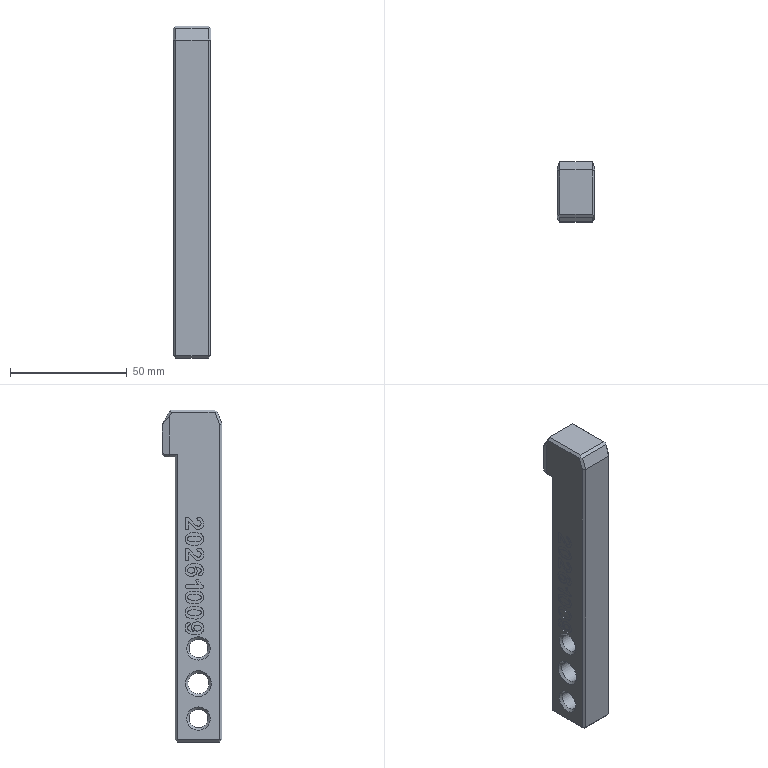Part | NX | features BREP 8, CHAMFER 2, solid 2, SUBTRACT 1 | 1 solid | 104 faces | box 16 x 25.5 x 142 mm | volume 43802 mm3 | plane 51 | spline 44 | cone 6 | cylinder 3 | commonest cylinder face diameters 8 x2 9 x1